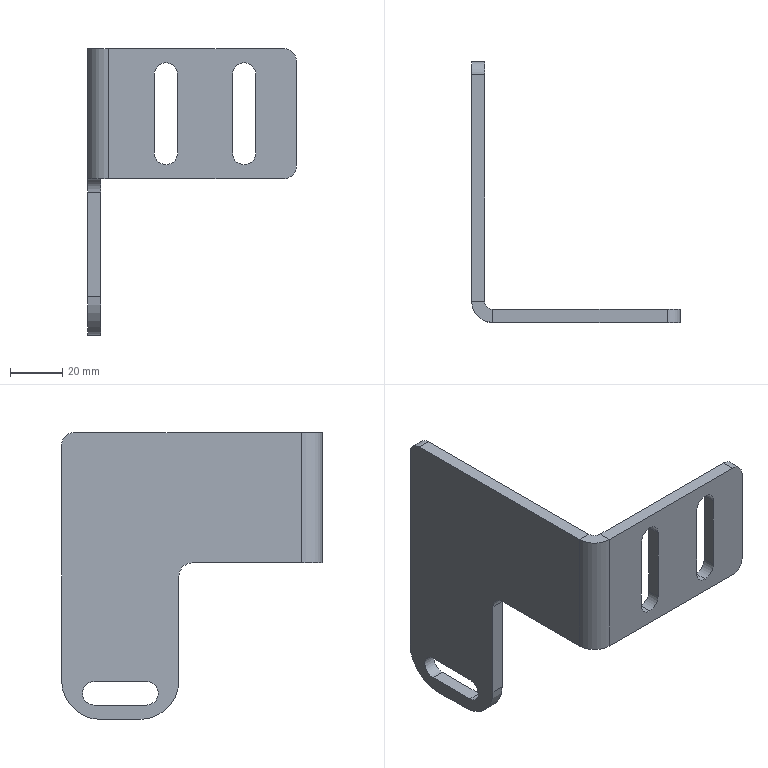Part | STEP file | 1 solid | 36 faces | box 80 x 100 x 110 mm | volume 51569 mm3 | plane 20 | cylinder 16 | commonest cylinder face diameters 9 x8 10 x4 30 x2 6 x1 16 x1